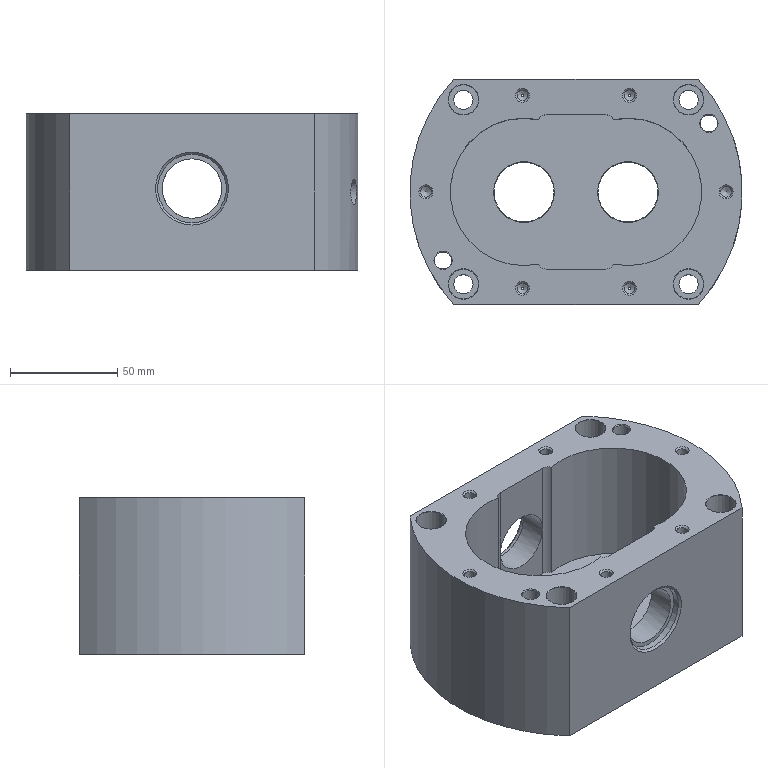NC program | NX | posted with a generic post | part box 155 x 105 x 73.2 mm
Lines 86 to 914 of 150882:
(HOLE_MILLING_COPY_COPY , TOOL : D10)
N146 T10 M6
N148 G54
N150 G17 G0 G90 X-24.25 Y0. B0. C0. S3000 M3
N152 G43 Z30. H10
N154 Z1.5
N156 G94 G3 X-25.5 Y1.25 R1.25 F2200.
N158 X-26.75 Y0. R1.25
N160 X-26.75 Y0. Z1.28 I2.5 J0.
N162 X-26.75 Y0. Z1.06 I2.5 J0.
N164 X-26.75 Y0. Z0.84 I2.5 J0.
N166 X-26.75 Y0. Z0.62 I2.5 J0.
N168 X-26.75 Y0. Z0.4 I2.5 J0.
N170 X-26.75 Y0. Z0.18 I2.5 J0.
N172 X-26.75 Y0. Z-0.04 I2.5 J0.
N174 X-26.75 Y0. Z-0.26 I2.5 J0.
N176 X-26.75 Y0. Z-0.48 I2.5 J0.
N178 X-26.75 Y0. Z-0.7 I2.5 J0.
N180 X-26.75 Y0. Z-0.92 I2.5 J0.
N182 X-26.75 Y0. Z-1.14 I2.5 J0.
N184 X-26.75 Y0. Z-1.36 I2.5 J0.
N186 X-26.75 Y0. Z-1.58 I2.5 J0.
N188 X-26.75 Y0. Z-1.8 I2.5 J0.
N190 X-26.75 Y0. Z-2.02 I2.5 J0.
N192 X-26.75 Y0. Z-2.24 I2.5 J0.
N194 X-26.75 Y0. Z-2.46 I2.5 J0.
N196 X-26.75 Y0. Z-2.68 I2.5 J0.
N198 X-26.75 Y0. Z-2.9 I2.5 J0.
N200 X-26.75 Y0. Z-3.12 I2.5 J0.
N202 X-26.75 Y0. Z-3.34 I2.5 J0.
N204 X-26.75 Y0. Z-3.56 I2.5 J0.
N206 X-26.75 Y0. Z-3.78 I2.5 J0.
N208 X-26.75 Y0. Z-4. I2.5 J0.
N210 X-26.75 Y0. Z-4.22 I2.5 J0.
N212 X-26.75 Y0. Z-4.44 I2.5 J0.
N214 X-26.75 Y0. Z-4.66 I2.5 J0.
N216 X-26.75 Y0. Z-4.88 I2.5 J0.
N218 X-26.75 Y0. Z-5.1 I2.5 J0.
N220 X-26.75 Y0. Z-5.32 I2.5 J0.
N222 X-26.75 Y0. Z-5.54 I2.5 J0.
N224 X-26.75 Y0. Z-5.76 I2.5 J0.
N226 X-26.75 Y0. Z-5.98 I2.5 J0.
N228 X-26.75 Y0. Z-6.2 I2.5 J0.
N230 X-26.75 Y0. Z-6.42 I2.5 J0.
N232 X-26.75 Y0. Z-6.64 I2.5 J0.
N234 X-26.75 Y0. Z-6.86 I2.5 J0.
N236 X-26.75 Y0. Z-7.08 I2.5 J0.
N238 X-26.75 Y0. Z-7.3 I2.5 J0.
N240 X-26.75 Y0. Z-7.52 I2.5 J0.
N242 X-26.75 Y0. Z-7.74 I2.5 J0.
N244 X-26.75 Y0. Z-7.96 I2.5 J0.
N246 X-26.75 Y0. Z-8.18 I2.5 J0.
N248 X-26.75 Y0. Z-8.4 I2.5 J0.
N250 X-26.75 Y0. Z-8.62 I2.5 J0.
N252 X-26.75 Y0. Z-8.84 I2.5 J0.
N254 X-26.75 Y0. Z-9.06 I2.5 J0.
N256 X-26.75 Y0. Z-9.28 I2.5 J0.
N258 X-26.75 Y0. Z-9.5 I2.5 J0.
N260 X-26.75 Y0. Z-9.72 I2.5 J0.
N262 X-26.75 Y0. Z-9.94 I2.5 J0.
N264 X-26.75 Y0. Z-10.16 I2.5 J0.
N266 X-26.75 Y0. Z-10.38 I2.5 J0.
N268 X-26.75 Y0. Z-10.6 I2.5 J0.
N270 X-26.75 Y0. Z-10.82 I2.5 J0.
N272 X-25.289 Y2.274 Z-11. R-2.5
N274 X-26.549 Y-1.067 R2.535
N276 X-23.204 Y-2.38 R2.565
N278 X-21.812 Y1.036 R2.617
N280 X-25.3 Y2.486 R2.681
N282 X-26.795 Y-1.039 R2.717
N284 X-23.199 Y-2.594 R2.78
N286 X-21.598 Y1.038 R2.817
N288 X-25.3 Y2.701 R2.88
N290 X-27.01 Y-1.036 R2.916
N292 X-23.204 Y-2.809 R2.979
N294 X-21.382 Y1.03 R3.016
N296 X-25.289 Y2.918 R3.079
N298 X-27.227 Y-1.021 R3.115
N300 X-23.222 Y-3.027 R3.179
N302 X-21.164 Y1.009 R3.215
N304 X-25.265 Y3.136 R3.278
N306 X-27.445 Y-0.995 R3.314
N308 X-23.251 Y-3.246 R3.378
N310 X-20.946 Y0.977 R3.414
N312 X-25.23 Y3.355 R3.477
N314 X-27.664 Y-0.957 R3.513
N316 X-23.292 Y-3.465 R3.577
N318 X-20.727 Y0.933 R3.613
N320 X-25.184 Y3.575 R3.676
N322 X-27.883 Y-0.907 R3.712
N324 X-23.344 Y-3.684 R3.776
N326 X-20.508 Y0.878 R3.812
N328 X-25.125 Y3.794 R3.875
N330 X-28.102 Y-0.845 R3.912
N332 X-23.409 Y-3.904 R3.975
N334 X-20.289 Y0.81 R4.011
N336 X-25.054 Y4.013 R4.074
N338 X-28.32 Y-0.772 R4.111
N340 X-23.485 Y-4.122 R4.174
N342 X-20.071 Y0.73 R4.21
N344 X-24.972 Y4.231 R4.274
N346 X-28.537 Y-0.686 R4.31
N348 X-23.574 Y-4.339 R4.373
N350 X-19.855 Y0.639 R4.409
N352 X-24.877 Y4.447 R4.473
N354 X-28.752 Y-0.589 R4.509
N356 X-23.674 Y-4.554 R4.572
N358 X-19.641 Y0.535 R4.608
N360 X-24.771 Y4.661 R4.672
N362 X-28.965 Y-0.479 R4.708
N364 X-23.786 Y-4.767 R4.771
N366 X-19.429 Y0.42 R4.807
N368 X-24.653 Y4.872 R4.871
N370 X-29.176 Y-0.358 R4.907
N372 X-23.91 Y-4.977 R4.97
N374 X-19.22 Y0.293 R5.007
N376 X-24.523 Y5.081 R5.07
N378 X-29.383 Y-0.225 R5.106
N380 X-24.046 Y-5.184 R5.169
N382 X-19.015 Y0.155 R5.206
N384 X-24.382 Y5.286 R5.269
N386 X-29.586 Y-0.081 R5.305
N388 X-24.194 Y-5.386 R5.369
N390 X-18.814 Y0.004 R5.405
N392 X-24.228 Y5.486 R5.468
N394 X-29.785 Y0.075 R5.504
N396 X-24.352 Y-5.585 R5.568
N398 X-18.617 Y-0.157 R5.604
N400 X-24.064 Y5.682 R5.667
N402 X-29.98 Y0.243 R5.703
N404 X-24.523 Y-5.778 R5.767
N406 X-18.425 Y-0.331 R5.803
N408 X-23.888 Y5.873 R5.866
N410 X-30.169 Y0.421 R5.902
N412 X-24.704 Y-5.967 R5.966
N414 X-18.238 Y-0.515 R6.002
N416 X-23.701 Y6.059 R6.065
N418 X-30.353 Y0.611 R6.101
N420 X-24.897 Y-6.149 R6.165
N422 X-18.058 Y-0.71 R6.201
N424 X-23.503 Y6.238 R6.264
N426 X-30.53 Y0.812 R6.301
N428 X-25.1 Y-6.325 R6.364
N430 X-17.884 Y-0.916 R6.4
N432 X-23.294 Y6.411 R6.464
N434 X-30.701 Y1.023 R6.5
N436 X-25.314 Y-6.495 R6.563
N438 X-17.717 Y-1.133 R6.599
N440 X-23.075 Y6.577 R6.663
N442 X-30.864 Y1.245 R6.699
N444 X-25.539 Y-6.657 R6.762
N446 X-17.557 Y-1.36 R6.798
N448 X-22.845 Y6.735 R6.862
N450 X-31.02 Y1.477 R6.898
N452 X-25.774 Y-6.811 R6.961
N454 X-17.405 Y-1.597 R6.997
N456 X-22.605 Y6.885 R7.061
N458 X-31.168 Y1.719 R7.097
N460 X-26.018 Y-6.957 R7.16
N462 X-17.261 Y-1.844 R7.196
N464 X-22.356 Y7.027 R7.26
N466 X-31.308 Y1.971 R7.296
N468 X-26.273 Y-7.095 R7.359
N470 X-17.126 Y-2.101 R7.396
N472 X-22.097 Y7.16 R7.459
N474 X-31.438 Y2.233 R7.495
N476 X-26.536 Y-7.223 R7.558
N478 X-17. Y-2.367 R7.595
N480 X-21.828 Y7.284 R7.658
N482 X-31.559 Y2.503 R7.694
N484 X-26.809 Y-7.342 R7.758
N486 X-16.884 Y-2.642 R7.794
N488 X-21.551 Y7.398 R7.857
N490 X-31.671 Y2.782 R7.893
N492 X-27.091 Y-7.452 R7.957
N494 X-16.778 Y-2.925 R7.993
N496 X-21.265 Y7.502 R8.056
N498 X-31.772 Y3.07 R8.092
N500 X-27.38 Y-7.551 R8.156
N502 X-16.682 Y-3.217 R8.192
N504 X-20.972 Y7.596 R8.255
N506 X-31.862 Y3.365 R8.291
N508 X-27.678 Y-7.639 R8.355
N510 X-16.596 Y-3.516 R8.391
N512 X-20.67 Y7.679 R8.454
N514 X-31.942 Y3.669 R8.49
N516 X-27.984 Y-7.716 R8.554
N518 X-16.522 Y-3.823 R8.59
N520 X-20.361 Y7.751 R8.653
N522 X-32.01 Y3.98 R8.69
N524 X-28.296 Y-7.782 R8.753
N526 X-16.46 Y-4.138 R8.789
N528 X-20.045 Y7.811 R8.853
N530 X-32.067 Y4.297 R8.889
N532 X-28.616 Y-7.836 R8.952
N534 X-16.409 Y-4.458 R8.988
N536 X-19.722 Y7.859 R9.052
N538 X-32.112 Y4.621 R9.088
N540 X-28.942 Y-7.878 R9.151
N542 X-16.37 Y-4.786 R9.187
N544 X-19.393 Y7.894 R9.251
N546 X-32.144 Y4.952 R9.287
N548 X-29.274 Y-7.908 R9.35
N550 X-16.344 Y-5.119 R9.386
N552 X-19.058 Y7.918 R9.45
N554 X-32.164 Y5.287 R9.486
N556 X-29.611 Y-7.924 R9.549
N558 X-16.331 Y-5.457 R9.585
N560 X-18.719 Y7.928 R9.649
N562 X-32.171 Y5.628 R9.685
N564 X-29.953 Y-7.928 R9.748
N566 X-16.331 Y-5.801 R9.785
N568 X-18.374 Y7.925 R9.848
N570 X-32.164 Y5.974 R9.884
N572 X-30.3 Y-7.919 R9.947
N574 X-16.344 Y-6.148 R9.984
N576 X-18.025 Y7.909 R10.047
N578 X-32.144 Y6.324 R10.083
N580 X-30.651 Y-7.896 R10.147
N582 X-16.371 Y-6.5 R10.183
N584 X-17.672 Y7.879 R10.246
N586 X-32.111 Y6.677 R10.282
N588 X-31.006 Y-7.859 R10.346
N590 X-16.411 Y-6.855 R10.382
N592 X-17.315 Y7.835 R10.445
N594 X-32.063 Y7.034 R10.481
N596 X-31.364 Y-7.808 R10.545
N598 X-16.466 Y-7.214 R10.581
N600 X-16.956 Y7.778 R10.644
N602 X-32.001 Y7.394 R10.68
N604 X-31.724 Y-7.743 R10.744
N606 X-16.535 Y-7.574 R10.78
N608 X-16.595 Y7.705 R10.843
N610 X-31.925 Y7.755 R10.879
N612 X-32.086 Y-7.664 R10.943
N614 X-16.618 Y-7.937 R10.979
N616 X-16.232 Y7.619 R11.042
N618 X-31.835 Y8.118 R11.079
N620 X-32.45 Y-7.57 R11.142
N622 X-16.716 Y-8.301 R11.178
N624 X-15.867 Y7.517 R11.242
N626 X-31.73 Y8.483 R11.278
N628 X-32.815 Y-7.461 R11.341
N630 X-16.829 Y-8.665 R11.377
N632 X-15.502 Y7.401 R11.441
N634 X-31.609 Y8.848 R11.477
N636 X-33.18 Y-7.338 R11.54
N638 X-16.956 Y-9.03 R11.576
N640 X-15.137 Y7.27 R11.64
N642 X-31.474 Y9.213 R11.676
N644 X-33.546 Y-7.199 R11.739
N646 X-17.099 Y-9.395 R11.775
N648 X-14.772 Y7.124 R11.839
N650 X-31.324 Y9.577 R11.875
N652 X-33.91 Y-7.046 R11.938
N654 X-17.256 Y-9.759 R11.974
N656 X-14.408 Y6.963 R12.038
N658 X-31.159 Y9.94 R12.074
N660 X-34.273 Y-6.877 R12.137
N662 X-17.429 Y-10.121 R12.174
N664 X-14.046 Y6.787 R12.237
N666 X-30.979 Y10.302 R12.273
N668 X-34.635 Y-6.693 R12.336
N670 X-17.617 Y-10.482 R12.373
N672 X-13.686 Y6.595 R12.436
N674 X-30.784 Y10.661 R12.472
N676 X-34.994 Y-6.494 R12.536
N678 X-17.82 Y-10.84 R12.572
N680 X-13.328 Y6.389 R12.635
N682 X-30.573 Y11.018 R12.671
N684 X-35.349 Y-6.28 R12.735
N686 X-18.038 Y-11.194 R12.771
N688 X-12.974 Y6.167 R12.834
N690 X-30.347 Y11.371 R12.87
N692 X-35.702 Y-6.05 R12.934
N694 X-18.272 Y-11.546 R12.97
N696 X-12.623 Y5.93 R13.033
N698 X-30.106 Y11.719 R13.069
N700 X-36.05 Y-5.806 R13.133
N702 X-18.52 Y-11.892 R13.169
N704 X-12.278 Y5.678 R13.232
N706 X-29.899 Y12.058 R13.284
N708 X-36.394 Y-5.546 R13.316
N710 X-18.704 Y-12.144 R13.35
N712 X-36.394 Y-5.546 R-13.35
N714 X-27.549 Y-8.845 R6.675
N716 X-24.25 Y0. R6.675
N718 G0 Z30.
N720 X24.25
N722 Z1.5
N724 G3 X23. Y1.25 R1.25
N726 X21.75 Y0. R1.25
N728 X21.75 Y0. Z1.28 I2.5 J0.
N730 X21.75 Y0. Z1.06 I2.5 J0.
N732 X21.75 Y0. Z0.84 I2.5 J0.
N734 X21.75 Y0. Z0.62 I2.5 J0.
N736 X21.75 Y0. Z0.4 I2.5 J0.
N738 X21.75 Y0. Z0.18 I2.5 J0.
N740 X21.75 Y0. Z-0.04 I2.5 J0.
N742 X21.75 Y0. Z-0.26 I2.5 J0.
N744 X21.75 Y0. Z-0.48 I2.5 J0.
N746 X21.75 Y0. Z-0.7 I2.5 J0.
N748 X21.75 Y0. Z-0.92 I2.5 J0.
N750 X21.75 Y0. Z-1.14 I2.5 J0.
N752 X21.75 Y0. Z-1.36 I2.5 J0.
N754 X21.75 Y0. Z-1.58 I2.5 J0.
N756 X21.75 Y0. Z-1.8 I2.5 J0.
N758 X21.75 Y0. Z-2.02 I2.5 J0.
N760 X21.75 Y0. Z-2.24 I2.5 J0.
N762 X21.75 Y0. Z-2.46 I2.5 J0.
N764 X21.75 Y0. Z-2.68 I2.5 J0.
N766 X21.75 Y0. Z-2.9 I2.5 J0.
N768 X21.75 Y0. Z-3.12 I2.5 J0.
N770 X21.75 Y0. Z-3.34 I2.5 J0.
N772 X21.75 Y0. Z-3.56 I2.5 J0.
N774 X21.75 Y0. Z-3.78 I2.5 J0.
N776 X21.75 Y0. Z-4. I2.5 J0.
N778 X21.75 Y0. Z-4.22 I2.5 J0.
N780 X21.75 Y0. Z-4.44 I2.5 J0.
N782 X21.75 Y0. Z-4.66 I2.5 J0.
N784 X21.75 Y0. Z-4.88 I2.5 J0.
N786 X21.75 Y0. Z-5.1 I2.5 J0.
N788 X21.75 Y0. Z-5.32 I2.5 J0.
N790 X21.75 Y0. Z-5.54 I2.5 J0.
N792 X21.75 Y0. Z-5.76 I2.5 J0.
N794 X21.75 Y0. Z-5.98 I2.5 J0.
N796 X21.75 Y0. Z-6.2 I2.5 J0.
N798 X21.75 Y0. Z-6.42 I2.5 J0.
N800 X21.75 Y0. Z-6.64 I2.5 J0.
N802 X21.75 Y0. Z-6.86 I2.5 J0.
N804 X21.75 Y0. Z-7.08 I2.5 J0.
N806 X21.75 Y0. Z-7.3 I2.5 J0.
N808 X21.75 Y0. Z-7.52 I2.5 J0.
N810 X21.75 Y0. Z-7.74 I2.5 J0.
N812 X21.75 Y0. Z-7.96 I2.5 J0.
N814 X21.75 Y0. Z-8.18 I2.5 J0.
N816 X21.75 Y0. Z-8.4 I2.5 J0.
N818 X21.75 Y0. Z-8.62 I2.5 J0.
N820 X21.75 Y0. Z-8.84 I2.5 J0.
N822 X21.75 Y0. Z-9.06 I2.5 J0.
N824 X21.75 Y0. Z-9.28 I2.5 J0.
N826 X21.75 Y0. Z-9.5 I2.5 J0.
N828 X21.75 Y0. Z-9.72 I2.5 J0.
N830 X21.75 Y0. Z-9.94 I2.5 J0.
N832 X21.75 Y0. Z-10.16 I2.5 J0.
N834 X21.75 Y0. Z-10.38 I2.5 J0.
N836 X21.75 Y0. Z-10.6 I2.5 J0.
N838 X21.75 Y0. Z-10.82 I2.5 J0.
N840 X23.211 Y2.274 Z-11. R-2.5
N842 X21.951 Y-1.067 R2.535
N844 X25.296 Y-2.38 R2.565
N846 X26.688 Y1.036 R2.617
N848 X23.2 Y2.486 R2.681
N850 X21.705 Y-1.039 R2.717
N852 X25.301 Y-2.594 R2.78
N854 X26.902 Y1.038 R2.817
N856 X23.2 Y2.701 R2.88
N858 X21.49 Y-1.036 R2.916
N860 X25.296 Y-2.809 R2.979
N862 X27.118 Y1.03 R3.016
N864 X23.211 Y2.918 R3.079
N866 X21.273 Y-1.021 R3.115
N868 X25.278 Y-3.027 R3.179
N870 X27.336 Y1.009 R3.215
N872 X23.235 Y3.136 R3.278
N874 X21.055 Y-0.995 R3.314
N876 X25.249 Y-3.246 R3.378
N878 X27.554 Y0.977 R3.414
N880 X23.27 Y3.355 R3.477
N882 X20.836 Y-0.957 R3.513
N884 X25.208 Y-3.465 R3.577
N886 X27.773 Y0.933 R3.613
N888 X23.316 Y3.575 R3.676
N890 X20.617 Y-0.907 R3.712
N892 X25.156 Y-3.684 R3.776
N894 X27.992 Y0.878 R3.812
N896 X23.375 Y3.794 R3.875
N898 X20.398 Y-0.845 R3.912
N900 X25.091 Y-3.904 R3.975
N902 X28.211 Y0.81 R4.011
N904 X23.446 Y4.013 R4.074
N906 X20.18 Y-0.772 R4.111
N908 X25.015 Y-4.122 R4.174
N910 X28.429 Y0.73 R4.21
N912 X23.528 Y4.231 R4.274
N914 X19.963 Y-0.686 R4.31
N916 X24.926 Y-4.339 R4.373
N918 X28.645 Y0.639 R4.409
N920 X23.623 Y4.447 R4.473
N922 X19.748 Y-0.589 R4.509
N924 X24.826 Y-4.554 R4.572
N926 X28.859 Y0.535 R4.608
N928 X23.729 Y4.661 R4.672
N930 X19.535 Y-0.479 R4.708
N932 X24.714 Y-4.767 R4.771
N934 X29.071 Y0.42 R4.807
N936 X23.847 Y4.872 R4.871
N938 X19.324 Y-0.358 R4.907
N940 X24.59 Y-4.977 R4.97
N942 X29.28 Y0.293 R5.007
N944 X23.977 Y5.081 R5.07
N946 X19.117 Y-0.225 R5.106
N948 X24.454 Y-5.184 R5.169
N950 X29.485 Y0.155 R5.206
N952 X24.118 Y5.286 R5.269
N954 X18.914 Y-0.081 R5.305
N956 X24.306 Y-5.386 R5.369
N958 X29.686 Y0.004 R5.405
N960 X24.272 Y5.486 R5.468
N962 X18.715 Y0.075 R5.504
N964 X24.148 Y-5.585 R5.568
N966 X29.883 Y-0.157 R5.604
N968 X24.436 Y5.682 R5.667
N970 X18.52 Y0.243 R5.703
N972 X23.977 Y-5.778 R5.767
N974 X30.075 Y-0.331 R5.803
N976 X24.612 Y5.873 R5.866
N978 X18.331 Y0.421 R5.902
N980 X23.796 Y-5.967 R5.966
N982 X30.262 Y-0.515 R6.002
N984 X24.799 Y6.059 R6.065
N986 X18.147 Y0.611 R6.101
N988 X23.603 Y-6.149 R6.165
N990 X30.442 Y-0.71 R6.201
N992 X24.997 Y6.238 R6.264
N994 X17.97 Y0.812 R6.301
N996 X23.4 Y-6.325 R6.364
N998 X30.616 Y-0.916 R6.4
N1000 X25.206 Y6.411 R6.464
N1002 X17.799 Y1.023 R6.5
N1004 X23.186 Y-6.495 R6.563
N1006 X30.783 Y-1.133 R6.599
N1008 X25.425 Y6.577 R6.663
N1010 X17.636 Y1.245 R6.699
N1012 X22.961 Y-6.657 R6.762
N1014 X30.943 Y-1.36 R6.798
N1016 X25.655 Y6.735 R6.862
N1018 X17.48 Y1.477 R6.898
N1020 X22.726 Y-6.811 R6.961
N1022 X31.095 Y-1.597 R6.997
N1024 X25.895 Y6.885 R7.061
N1026 X17.332 Y1.719 R7.097
N1028 X22.482 Y-6.957 R7.16
N1030 X31.239 Y-1.844 R7.196
N1032 X26.144 Y7.027 R7.26
N1034 X17.192 Y1.971 R7.296
N1036 X22.227 Y-7.095 R7.359
N1038 X31.374 Y-2.101 R7.396
N1040 X26.403 Y7.16 R7.459
N1042 X17.062 Y2.233 R7.495
N1044 X21.964 Y-7.223 R7.558
N1046 X31.5 Y-2.367 R7.595
N1048 X26.672 Y7.284 R7.658
N1050 X16.941 Y2.503 R7.694
N1052 X21.691 Y-7.342 R7.758
N1054 X31.616 Y-2.642 R7.794
N1056 X26.949 Y7.398 R7.857
N1058 X16.829 Y2.782 R7.893
N1060 X21.409 Y-7.452 R7.957
N1062 X31.722 Y-2.925 R7.993
N1064 X27.235 Y7.502 R8.056
N1066 X16.728 Y3.07 R8.092
N1068 X21.12 Y-7.551 R8.156
N1070 X31.818 Y-3.217 R8.192
N1072 X27.528 Y7.596 R8.255
N1074 X16.638 Y3.365 R8.291
N1076 X20.822 Y-7.639 R8.355
N1078 X31.904 Y-3.516 R8.391
N1080 X27.83 Y7.679 R8.454
N1082 X16.558 Y3.669 R8.49
N1084 X20.516 Y-7.716 R8.554
N1086 X31.978 Y-3.823 R8.59
N1088 X28.139 Y7.751 R8.653
N1090 X16.49 Y3.98 R8.69
N1092 X20.204 Y-7.782 R8.753
N1094 X32.04 Y-4.138 R8.789
N1096 X28.455 Y7.811 R8.853
N1098 X16.433 Y4.297 R8.889
N1100 X19.884 Y-7.836 R8.952
N1102 X32.091 Y-4.458 R8.988
N1104 X28.778 Y7.859 R9.052
N1106 X16.388 Y4.621 R9.088
N1108 X19.558 Y-7.878 R9.151
N1110 X32.13 Y-4.786 R9.187
N1112 X29.107 Y7.894 R9.251
N1114 X16.356 Y4.952 R9.287
N1116 X19.226 Y-7.908 R9.35
N1118 X32.156 Y-5.119 R9.386
N1120 X29.442 Y7.918 R9.45
N1122 X16.336 Y5.287 R9.486
N1124 X18.889 Y-7.924 R9.549
N1126 X32.169 Y-5.457 R9.585
N1128 X29.781 Y7.928 R9.649
N1130 X16.329 Y5.628 R9.685
N1132 X18.547 Y-7.928 R9.748
N1134 X32.169 Y-5.801 R9.785
N1136 X30.126 Y7.925 R9.848
N1138 X16.336 Y5.974 R9.884
N1140 X18.2 Y-7.919 R9.947
N1142 X32.156 Y-6.148 R9.984
N1144 X30.475 Y7.909 R10.047
N1146 X16.356 Y6.324 R10.083
N1148 X17.849 Y-7.896 R10.147
N1150 X32.129 Y-6.5 R10.183
N1152 X30.828 Y7.879 R10.246
N1154 X16.389 Y6.677 R10.282
N1156 X17.494 Y-7.859 R10.346
N1158 X32.089 Y-6.855 R10.382
N1160 X31.185 Y7.835 R10.445
N1162 X16.437 Y7.034 R10.481
N1164 X17.136 Y-7.808 R10.545
N1166 X32.034 Y-7.214 R10.581
N1168 X31.544 Y7.778 R10.644
N1170 X16.499 Y7.394 R10.68
N1172 X16.776 Y-7.743 R10.744
N1174 X31.965 Y-7.574 R10.78
N1176 X31.905 Y7.705 R10.843
N1178 X16.575 Y7.755 R10.879
N1180 X16.414 Y-7.664 R10.943
N1182 X31.882 Y-7.937 R10.979
N1184 X32.268 Y7.619 R11.042
N1186 X16.665 Y8.118 R11.079
N1188 X16.05 Y-7.57 R11.142
N1190 X31.784 Y-8.301 R11.178
N1192 X32.633 Y7.517 R11.242
N1194 X16.77 Y8.483 R11.278
N1196 X15.685 Y-7.461 R11.341
N1198 X31.671 Y-8.665 R11.377
N1200 X32.998 Y7.401 R11.441
N1202 X16.891 Y8.848 R11.477
N1204 X15.32 Y-7.338 R11.54
N1206 X31.544 Y-9.03 R11.576
N1208 X33.363 Y7.27 R11.64
N1210 X17.026 Y9.213 R11.676
N1212 X14.954 Y-7.199 R11.739
N1214 X31.401 Y-9.395 R11.775
N1216 X33.728 Y7.124 R11.839
N1218 X17.176 Y9.577 R11.875
N1220 X14.59 Y-7.046 R11.938
N1222 X31.244 Y-9.759 R11.974
N1224 X34.092 Y6.963 R12.038
N1226 X17.341 Y9.94 R12.074
N1228 X14.227 Y-6.877 R12.137
N1230 X31.071 Y-10.121 R12.174
N1232 X34.454 Y6.787 R12.237
N1234 X17.521 Y10.302 R12.273
N1236 X13.865 Y-6.693 R12.336
N1238 X30.883 Y-10.482 R12.373
N1240 X34.814 Y6.595 R12.436
N1242 X17.716 Y10.661 R12.472
N1244 X13.506 Y-6.494 R12.536
N1246 X30.68 Y-10.84 R12.572
N1248 X35.172 Y6.389 R12.635
N1250 X17.927 Y11.018 R12.671
N1252 X13.151 Y-6.28 R12.735
N1254 X30.462 Y-11.194 R12.771
N1256 X35.526 Y6.167 R12.834
N1258 X18.153 Y11.371 R12.87
N1260 X12.798 Y-6.05 R12.934
N1262 X30.228 Y-11.546 R12.97
N1264 X35.877 Y5.93 R13.033
N1266 X18.394 Y11.719 R13.069
N1268 X12.45 Y-5.806 R13.133
N1270 X29.98 Y-11.892 R13.169
N1272 X36.222 Y5.678 R13.232
N1274 X18.601 Y12.058 R13.284
N1276 X12.106 Y-5.546 R13.316
N1278 X29.796 Y-12.144 R13.35
N1280 X12.106 Y-5.546 R-13.35
N1282 X20.951 Y-8.845 R6.675
N1284 X24.25 Y0. R6.675
N1286 G0 Z30.
(HOLE_MILLING_COPY_COPY_COPY , TOOL : D10)
N1288 X-24.25
N1290 Z-10.
N1292 G3 X-25.5 Y1.25 R1.25
N1294 X-26.75 Y0. R1.25
N1296 X-26.75 Y0. Z-10.22 I2.5 J0.
N1298 X-26.75 Y0. Z-10.44 I2.5 J0.
N1300 X-26.75 Y0. Z-10.66 I2.5 J0.
N1302 X-26.75 Y0. Z-10.88 I2.5 J0.
N1304 X-26.75 Y0. Z-11.1 I2.5 J0.
N1306 X-26.75 Y0. Z-11.32 I2.5 J0.
N1308 X-26.75 Y0. Z-11.54 I2.5 J0.
N1310 X-26.75 Y0. Z-11.76 I2.5 J0.
N1312 X-26.75 Y0. Z-11.98 I2.5 J0.
N1314 X-26.75 Y0. Z-12.2 I2.5 J0.
N1316 X-26.75 Y0. Z-12.42 I2.5 J0.
N1318 X-26.75 Y0. Z-12.64 I2.5 J0.
N1320 X-26.75 Y0. Z-12.86 I2.5 J0.
N1322 X-26.75 Y0. Z-13.08 I2.5 J0.
N1324 X-26.75 Y0. Z-13.3 I2.5 J0.
N1326 X-26.75 Y0. Z-13.52 I2.5 J0.
N1328 X-26.75 Y0. Z-13.74 I2.5 J0.
N1330 X-26.75 Y0. Z-13.96 I2.5 J0.
N1332 X-25.289 Y-2.274 Z-14. R2.5
N1334 X-21.93 Y-1.022 R2.534
N1336 X-23.17 Y2.365 R2.566
N1338 X-26.655 Y1.113 R2.618
N1340 X-25.372 Y-2.456 R2.682
N1342 X-21.754 Y-1.155 R2.718
N1344 X-23.087 Y2.547 R2.782
N1346 X-26.837 Y1.196 R2.818
N1348 X-25.455 Y-2.638 R2.882
N1350 X-21.572 Y-1.238 R2.918
N1352 X-23.004 Y2.729 R2.982
N1354 X-27.019 Y1.279 R3.018
N1356 X-25.538 Y-2.82 R3.082
N1358 X-21.39 Y-1.321 R3.118
N1360 X-22.921 Y2.911 R3.182
N1362 X-27.201 Y1.362 R3.218
N1364 X-25.621 Y-3.002 R3.282
N1366 X-21.209 Y-1.404 R3.318
N1368 X-22.838 Y3.093 R3.382
N1370 X-27.382 Y1.446 R3.418
N1372 X-25.704 Y-3.184 R3.482
N1374 X-21.027 Y-1.487 R3.518
N1376 X-22.755 Y3.275 R3.582
N1378 X-27.564 Y1.529 R3.618
N1380 X-25.787 Y-3.366 R3.682
N1382 X-20.845 Y-1.57 R3.718
N1384 X-22.671 Y3.457 R3.782
N1386 X-27.746 Y1.612 R3.818
N1388 X-25.87 Y-3.548 R3.882
N1390 X-20.663 Y-1.653 R3.918
N1392 X-22.588 Y3.639 R3.982
N1394 X-27.928 Y1.695 R4.018
N1396 X-25.953 Y-3.729 R4.082
N1398 X-20.481 Y-1.736 R4.118
N1400 X-22.505 Y3.82 R4.182
N1402 X-28.11 Y1.778 R4.218
N1404 X-26.036 Y-3.911 R4.282
N1406 X-20.299 Y-1.819 R4.318
N1408 X-22.422 Y4.002 R4.382
N1410 X-28.292 Y1.861 R4.418
N1412 X-26.119 Y-4.093 R4.482
N1414 X-20.117 Y-1.903 R4.518
N1416 X-22.339 Y4.184 R4.582
N1418 X-28.474 Y1.944 R4.618
N1420 X-26.202 Y-4.275 R4.682
N1422 X-19.935 Y-1.986 R4.718
N1424 X-22.256 Y4.366 R4.782
N1426 X-28.656 Y2.027 R4.818
N1428 X-26.286 Y-4.457 R4.882
N1430 X-19.753 Y-2.069 R4.918
N1432 X-22.173 Y4.548 R4.982
N1434 X-28.838 Y2.11 R5.018
N1436 X-26.369 Y-4.639 R5.082
N1438 X-19.571 Y-2.152 R5.118
N1440 X-22.09 Y4.73 R5.182
N1442 X-29.02 Y2.193 R5.218
N1444 X-26.452 Y-4.821 R5.282
N1446 X-19.389 Y-2.235 R5.318
N1448 X-22.007 Y4.912 R5.382
N1450 X-29.202 Y2.276 R5.418
N1452 X-26.535 Y-5.003 R5.482
N1454 X-19.207 Y-2.318 R5.518
N1456 X-21.924 Y5.094 R5.582
N1458 X-29.384 Y2.359 R5.618
N1460 X-26.618 Y-5.185 R5.682
N1462 X-19.025 Y-2.401 R5.718
N1464 X-21.841 Y5.276 R5.782
N1466 X-29.566 Y2.443 R5.818
N1468 X-26.701 Y-5.367 R5.882
N1470 X-18.843 Y-2.484 R5.918
N1472 X-21.758 Y5.458 R5.982
N1474 X-29.748 Y2.526 R6.018
N1476 X-26.784 Y-5.549 R6.082
N1478 X-18.662 Y-2.567 R6.118
N1480 X-21.674 Y5.64 R6.182
N1482 X-29.929 Y2.609 R6.218
N1484 X-26.867 Y-5.731 R6.282
N1486 X-18.48 Y-2.65 R6.318
N1488 X-21.591 Y5.822 R6.382
N1490 X-30.111 Y2.692 R6.418
N1492 X-26.95 Y-5.913 R6.482
N1494 X-18.298 Y-2.733 R6.518
N1496 X-21.508 Y6.004 R6.582
N1498 X-30.293 Y2.775 R6.618
N1500 X-27.033 Y-6.095 R6.682
N1502 X-18.116 Y-2.816 R6.718
N1504 X-21.425 Y6.185 R6.782
N1506 X-30.475 Y2.858 R6.818
N1508 X-27.116 Y-6.276 R6.882
N1510 X-17.934 Y-2.9 R6.918
N1512 X-21.342 Y6.367 R6.982
N1514 X-30.657 Y2.941 R7.018
N1516 X-27.199 Y-6.458 R7.082
N1518 X-17.752 Y-2.983 R7.118
N1520 X-21.259 Y6.549 R7.182
N1522 X-30.839 Y3.024 R7.218
N1524 X-27.283 Y-6.64 R7.282
N1526 X-17.57 Y-3.066 R7.318
N1528 X-21.176 Y6.731 R7.382
N1530 X-31.021 Y3.107 R7.418
N1532 X-27.366 Y-6.822 R7.482
N1534 X-17.388 Y-3.149 R7.518
N1536 X-21.093 Y6.913 R7.582
N1538 X-31.203 Y3.19 R7.618
N1540 X-27.449 Y-7.004 R7.682
N1542 X-17.206 Y-3.232 R7.718
N1544 X-21.01 Y7.095 R7.782
N1546 X-31.385 Y3.273 R7.818
N1548 X-27.532 Y-7.186 R7.882
N1550 X-17.024 Y-3.315 R7.918
N1552 X-20.927 Y7.277 R7.982
N1554 X-31.567 Y3.356 R8.018
N1556 X-27.615 Y-7.368 R8.082
N1558 X-16.842 Y-3.398 R8.118
N1560 X-20.844 Y7.459 R8.182
N1562 X-31.749 Y3.44 R8.218
N1564 X-27.698 Y-7.55 R8.282
N1566 X-16.66 Y-3.481 R8.318
N1568 X-20.761 Y7.641 R8.382
N1570 X-31.931 Y3.523 R8.418
N1572 X-27.781 Y-7.732 R8.482
N1574 X-16.478 Y-3.564 R8.518
N1576 X-20.677 Y7.823 R8.582
N1578 X-32.113 Y3.606 R8.618
N1580 X-27.864 Y-7.914 R8.682
N1582 X-16.296 Y-3.647 R8.718
N1584 X-20.594 Y8.005 R8.782
N1586 X-32.329 Y3.652 R8.834
N1588 X-27.947 Y-8.096 R8.866
N1590 X-16.154 Y-3.697 R8.9
N1592 X-27.947 Y-8.096 R-8.9
N1594 X-22.051 Y-5.896 R4.45
N1596 X-24.25 Y0. R4.45
N1598 G0 Z30.
N1600 X24.25
N1602 Z-10.
N1604 G3 X23. Y1.25 R1.25
N1606 X21.75 Y0. R1.25
N1608 X21.75 Y0. Z-10.22 I2.5 J0.
N1610 X21.75 Y0. Z-10.44 I2.5 J0.
N1612 X21.75 Y0. Z-10.66 I2.5 J0.
N1614 X21.75 Y0. Z-10.88 I2.5 J0.
N1616 X21.75 Y0. Z-11.1 I2.5 J0.
N1618 X21.75 Y0. Z-11.32 I2.5 J0.
N1620 X21.75 Y0. Z-11.54 I2.5 J0.
N1622 X21.75 Y0. Z-11.76 I2.5 J0.
N1624 X21.75 Y0. Z-11.98 I2.5 J0.
N1626 X21.75 Y0. Z-12.2 I2.5 J0.
N1628 X21.75 Y0. Z-12.42 I2.5 J0.
N1630 X21.75 Y0. Z-12.64 I2.5 J0.
N1632 X21.75 Y0. Z-12.86 I2.5 J0.
N1634 X21.75 Y0. Z-13.08 I2.5 J0.
N1636 X21.75 Y0. Z-13.3 I2.5 J0.
N1638 X21.75 Y0. Z-13.52 I2.5 J0.
N1640 X21.75 Y0. Z-13.74 I2.5 J0.
N1642 X21.75 Y0. Z-13.96 I2.5 J0.
N1644 X23.211 Y-2.274 Z-14. R2.5
N1646 X26.57 Y-1.022 R2.534
N1648 X25.33 Y2.365 R2.566
N1650 X21.845 Y1.113 R2.618
N1652 X23.128 Y-2.456 R2.682
N1654 X26.746 Y-1.155 R2.718
N1656 X25.413 Y2.547 R2.782
N1658 X21.663 Y1.196 R2.818
N1660 X23.045 Y-2.638 R2.882
N1662 X26.928 Y-1.238 R2.918
N1664 X25.496 Y2.729 R2.982
N1666 X21.481 Y1.279 R3.018
N1668 X22.962 Y-2.82 R3.082
N1670 X27.11 Y-1.321 R3.118
N1672 X25.579 Y2.911 R3.182
N1674 X21.299 Y1.362 R3.218
N1676 X22.879 Y-3.002 R3.282
N1678 X27.291 Y-1.404 R3.318
N1680 X25.662 Y3.093 R3.382
N1682 X21.118 Y1.446 R3.418
N1684 X22.796 Y-3.184 R3.482
N1686 X27.473 Y-1.487 R3.518
N1688 X25.745 Y3.275 R3.582
N1690 X20.936 Y1.529 R3.618
N1692 X22.713 Y-3.366 R3.682
N1694 X27.655 Y-1.57 R3.718
N1696 X25.829 Y3.457 R3.782
N1698 X20.754 Y1.612 R3.818
N1700 X22.63 Y-3.548 R3.882
N1702 X27.837 Y-1.653 R3.918
N1704 X25.912 Y3.639 R3.982
N1706 X20.572 Y1.695 R4.018
N1708 X22.547 Y-3.729 R4.082
N1710 X28.019 Y-1.736 R4.118
N1712 X25.995 Y3.82 R4.182
N1714 X20.39 Y1.778 R4.218
N1716 X22.464 Y-3.911 R4.282
N1718 X28.201 Y-1.819 R4.318
N1720 X26.078 Y4.002 R4.382
N1722 X20.208 Y1.861 R4.418
N1724 X22.381 Y-4.093 R4.482
N1726 X28.383 Y-1.903 R4.518
N1728 X26.161 Y4.184 R4.582
N1730 X20.026 Y1.944 R4.618
N1732 X22.298 Y-4.275 R4.682
N1734 X28.565 Y-1.986 R4.718
N1736 X26.244 Y4.366 R4.782
N1738 X19.844 Y2.027 R4.818
N1740 X22.214 Y-4.457 R4.882
N1742 X28.747 Y-2.069 R4.918
N1744 X26.327 Y4.548 R4.982
N1746 X19.662 Y2.11 R5.018
N1748 X22.131 Y-4.639 R5.082
N1750 X28.929 Y-2.152 R5.118
N1752 X26.41 Y4.73 R5.182
N1754 X19.48 Y2.193 R5.218
N1756 X22.048 Y-4.821 R5.282
N1758 X29.111 Y-2.235 R5.318
N1760 X26.493 Y4.912 R5.382
N1762 X19.298 Y2.276 R5.418
N1764 X21.965 Y-5.003 R5.482
N1766 X29.293 Y-2.318 R5.518
N1768 X26.576 Y5.094 R5.582
N1770 X19.116 Y2.359 R5.618
N1772 X21.882 Y-5.185 R5.682
N1774 X29.475 Y-2.401 R5.718
N1776 X26.659 Y5.276 R5.782
N1778 X18.934 Y2.443 R5.818
N1780 X21.799 Y-5.367 R5.882
N1782 X29.657 Y-2.484 R5.918
N1784 X26.742 Y5.458 R5.982
N1786 X18.752 Y2.526 R6.018
N1788 X21.716 Y-5.549 R6.082
N1790 X29.838 Y-2.567 R6.118